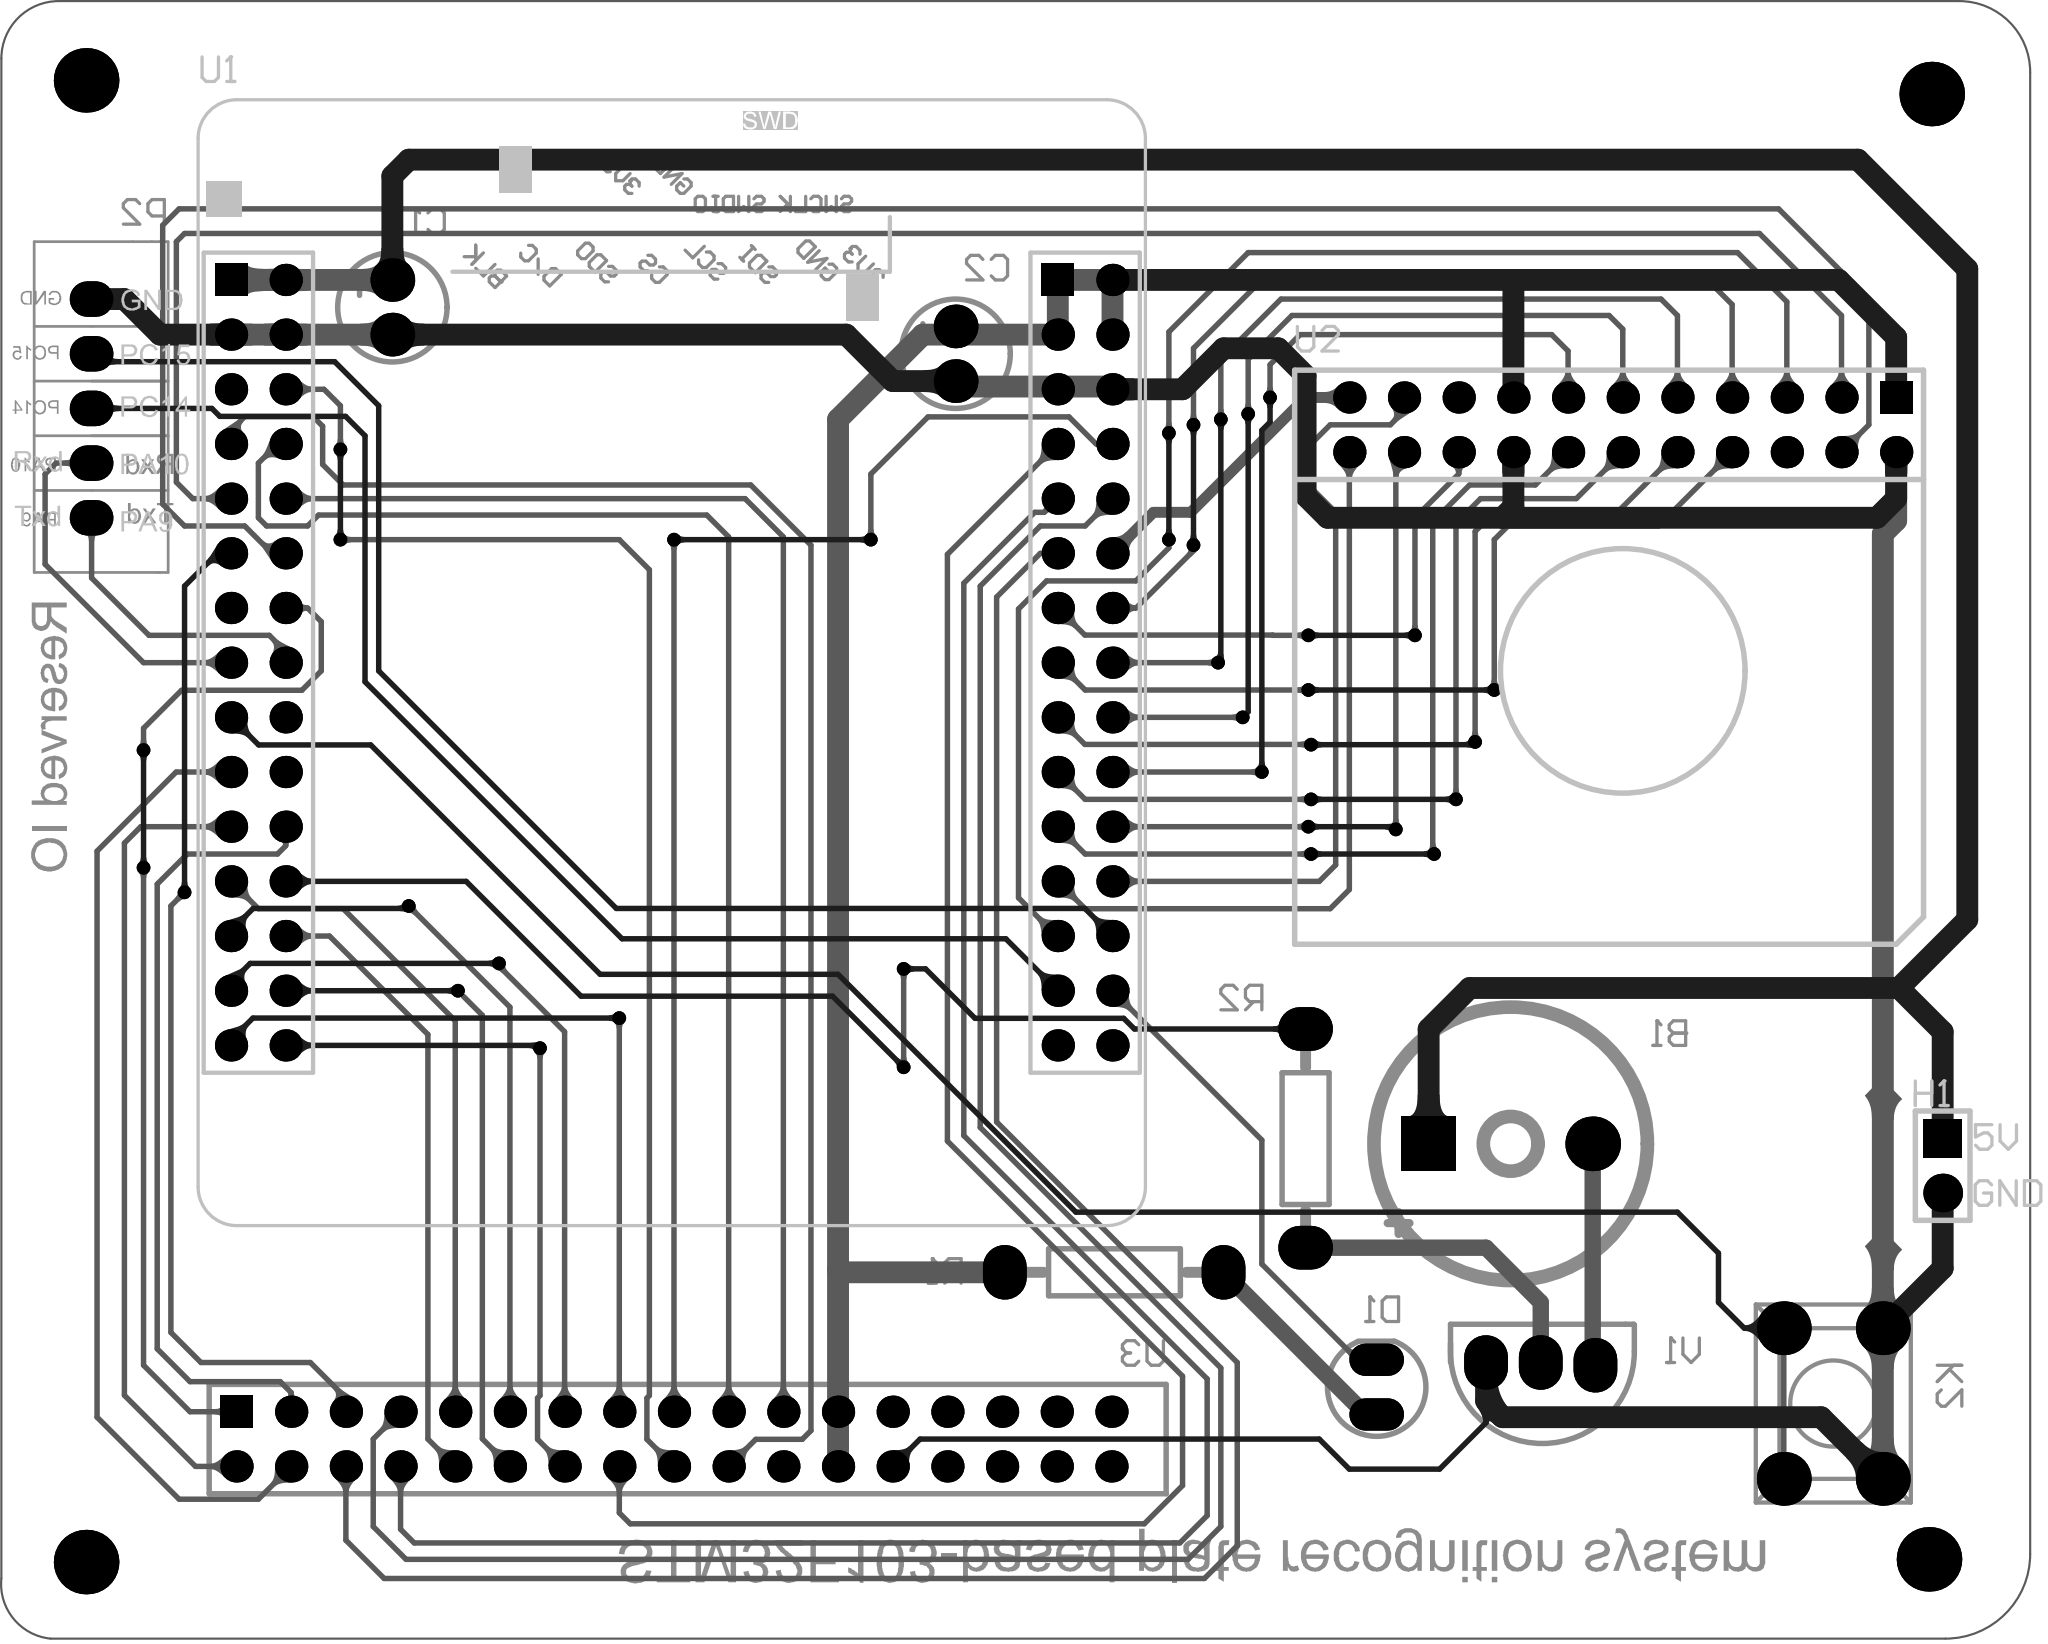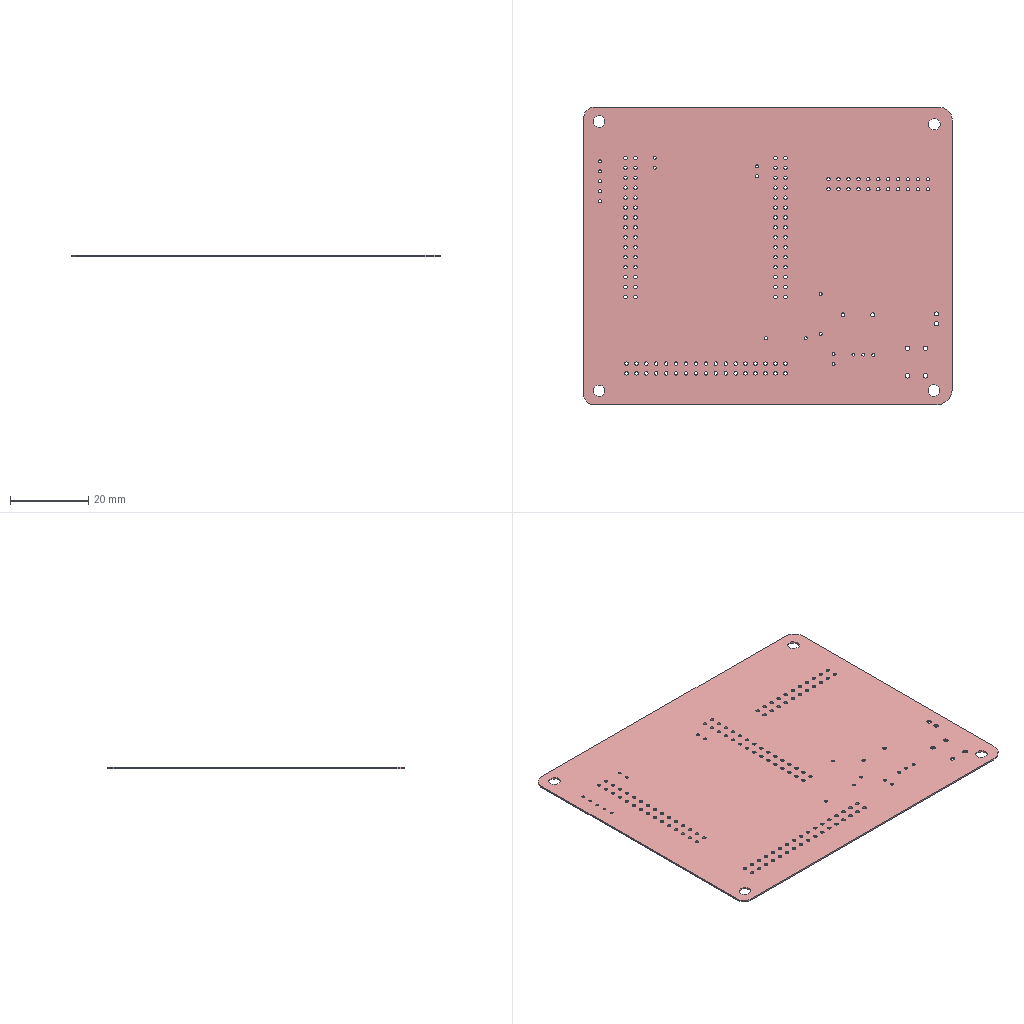Circuit board layout | Altium Designer | box 94.2 x 76.1 x 0.4 mm
Layer stack:
# Altium Designer layer stack of  (unit mm; dielectric type: 0 none, 1 core, 2 prepreg, 3 surface material)
index,name,kind,layer,copper_thickness_mm,dielectric_type,dielectric_thickness_mm,dielectric_material,dielectric_constant
0,Top Paste Mask Layer,other,,,,,,
1,Top Silkscreen Layer,other,,,,,,
2,Top Solder Mask Layer,dielectric,,,3,0.0102,Solder Resist,3.5
3,Top Layer,copper,Top Layer,0.0356,,,,
4,Dielectric1,dielectric,,,3,0.32,FR-4,4.8
5,Bottom Layer,copper,Bottom Layer,0.0356,,,,
6,Bottom Solder Mask Layer,dielectric,,,3,0.0102,Solder Resist,3.5
7,Bottom Silkscreen Layer,other,,,,,,
8,Bottom Paste Mask Layer,other,,,,,,
# drill layer pairs: low layer,high layer
drill_pair,Top Layer,Bottom Layer
Part placement:
Designator,Comment,Layer,Footprint,Center-X(mm),Center-Y(mm),Rotation
B1,Buzzer FMQ,BottomLayer,蜂鸣器,146.317,99.187,0
C1,10uf,BottomLayer,CD0.254cm,94.374,138.049,270
C2,10uf,BottomLayer,CD0.254cm,120.536,135.89,270
D1,LED,BottomLayer,发光二极管FZ,140.094,87.884,90
H1,,TopLayer,HDR-TH_2P-P2.54-V-M-1,166.383,98.171,270
K2,Key button,BottomLayer,按键,161.303,87.122,270
P2,5P,BottomLayer,5ZHEN-100mil,80.404,133.35,0
R1,1K,BottomLayer,电阻FZ,127.902,93.218,0
R2,10K,BottomLayer,电阻FZ,136.792,99.441,270
U1,STM32F103RCT6 core board,TopLayer,STM32F103RC/RB_ºËÐÄ°å,107.351,121.539,0
U2,OV7670 with FIFO,TopLayer,OV7670模块,151.524,132.588,180
U3,TFT_ILI9341 2.8,BottomLayer,2.8寸TFT,107.455,85.471,0
V1,Transistor 3,BottomLayer,三极管FZ,147.714,88.963,0
Pad and via stacks:
# Altium Designer via and pad stacks of  (unit mm). Each distinct definition once, with the count of objects using it.
# via: kind,start_layer,end_layer,hole_mm,diameter_mm,mode(0 simple;1 top-mid-bottom;2 full stack),diameter_per_layer,count,example_net
# pad: kind,layer,hole_mm,hole_type(0 round;1 square;2 slot),plating,top_size,top_shape(1 round;2 rect;3 octagon;9 rounded rect),mid_size,bottom_size,mode,footprint,size_per_layer,count,example
pad,Multi-Layer,3,0,plated,3x3,1,3x3,3x3,0,,,4,
pad,Multi-Layer,1.016,0,plated,2.54x2.54,1,2.54x2.54,2.54x2.54,0,\u00B7\u00E4\u00C3\u00F9\u00C6\u00F7,,1,B1.2
pad,Multi-Layer,1.016,0,plated,2.54x2.54,2,2.54x2.54,2.54x2.54,0,\u00B7\u00E4\u00C3\u00F9\u00C6\u00F7,,1,B1.1
pad,Multi-Layer,0.762,0,plated,2.032x2.032,1,2.032x2.032,2.032x2.032,0,CD0.254cm,,4,C1.2
pad,Multi-Layer,0.762,0,plated,1.5x2.54,1,1.5x2.54,1.5x2.54,0,\u00B7\u00A2\u00B9\u00E2\u00B6\u00FE\u00BC\u00AB\u00B9\u00DCFZ,,2,D1.1
pad,Multi-Layer,1.1,0,plated,1.8x1.8,1,1.8x1.8,1.8x1.8,0,HDR-TH_2P-P2.54-V-M-1,,1,H1.2
pad,Multi-Layer,1.1,0,plated,1.8x1.8,2,1.8x1.8,1.8x1.8,0,HDR-TH_2P-P2.54-V-M-1,,1,H1.1
pad,Multi-Layer,1.2,0,plated,2.5x2.5,1,2.5x2.5,2.5x2.5,0,\u00B0\u00B4\u00BC\u00FC,,4,K2.1
pad,Multi-Layer,0.762,0,plated,2.032x1.651,1,2.032x1.651,2.032x1.651,0,5ZHEN-100mil,,5,P2.1
pad,Multi-Layer,0.762,0,plated,2.54x2.032,1,2.54x2.032,2.54x2.032,0,\u00B5\u00E7\u00D7\u00E8FZ,,4,R1.2
pad,Multi-Layer,0.9,0,plated,1.5x1.5,2,1.5x1.5,1.5x1.5,0,STM32F103RC/RB \u00BA\u00CB\u00D0\u00C4\u00B0\u00E5,,2,U1.1
pad,Multi-Layer,0.9,0,plated,1.5x1.5,1,1.5x1.5,1.5x1.5,0,STM32F103RC/RB \u00BA\u00CB\u00D0\u00C4\u00B0\u00E5,,58,U1.2
pad,Multi-Layer,0.9,0,plated,1.5x1.5,1,1.5x1.5,1.5x1.5,0,OV7670\u00C4\u00A3\u00BF\u00E9,,21,U2.22
pad,Multi-Layer,0.9,0,plated,1.5x1.5,2,1.5x1.5,1.5x1.5,0,OV7670\u00C4\u00A3\u00BF\u00E9,,1,U2.1
pad,Multi-Layer,0.9,0,plated,1.5x1.5,1,1.5x1.5,1.5x1.5,0,2.8\u00B4\u00E7TFT,,33,U3.34
pad,Multi-Layer,0.9,0,plated,1.5x1.5,2,1.5x1.5,1.5x1.5,0,2.8\u00B4\u00E7TFT,,1,U3.1
pad,Multi-Layer,0.762,0,plated,2.54x2.032,1,2.54x2.032,2.54x2.032,0,\u00C8\u00FD\u00BC\u00AB\u00B9\u00DCFZ,,2,V1.1
pad,Multi-Layer,0.762,0,plated,2.032x2.54,1,2.032x2.54,2.032x2.54,0,\u00C8\u00FD\u00BC\u00AB\u00B9\u00DCFZ,,1,V1.2
via,Top Layer,Bottom Layer,0.381,0.635,0,,36,PB8
Design rules, without the lines most boards share:
# Altium Designer design rules of  (exported by Altium Designer, unit mm)
# columns: name | kind | enabled | priority | scope1 | scope2 | descriptor | typed fields (field=value)
Plane_innerPlane | 0 | disabled | 1 | All | All | Clearance Constraint (Gap=6mil) (Disabled)(All),(All) | gap=0.1524
Plane_innerPlane_1 | 63 | disabled | 1 | All | All | Board Clearance Constraint (Gap=0mil) (Disabled)(All) |
Copper_copperRegion | 0 | disabled | 2 | All | All | Clearance Constraint (Gap=6mil) (Disabled)(All),(All) | gap=0.1524
Copper_copperRegion_1 | 63 | disabled | 2 | All | All | Board Clearance Constraint (Gap=0mil) (Disabled)(All) |
safeClearance | 0 | enabled | 3 | All | All | Clearance Constraint (Gap=6mil) (All),(All) | gap=0.1524
safeClearance_1 | 63 | enabled | 3 | All | All | Board Clearance Constraint (Gap=0mil) (All) |
HoleToHoleClearance | 52 | enabled | 1 | All | All | Hole To Hole Clearance (Gap=10mil) (All),(All) | gap=0.254
trackWidth | 2 | enabled | 1 | All | All | Width Constraint (Min=5mil) (Max=100mil) (Preferred=10mil) (All) |
viaSize | 11 | enabled | 1 | All | All | Routing Via (MinHoleWidth=11.811mil) (MaxHoleWidth=236.22mil) (PreferredHoleWidth=12.008mil) (MinWidth=19.685mil) (MaxWidth=393.701mil) (PreferedWidth=24.016mil) (All) | via_min_hole=0.3 via_max_hole=6 via_preferred_diameter=0.61 via_preferred_hole=0.305